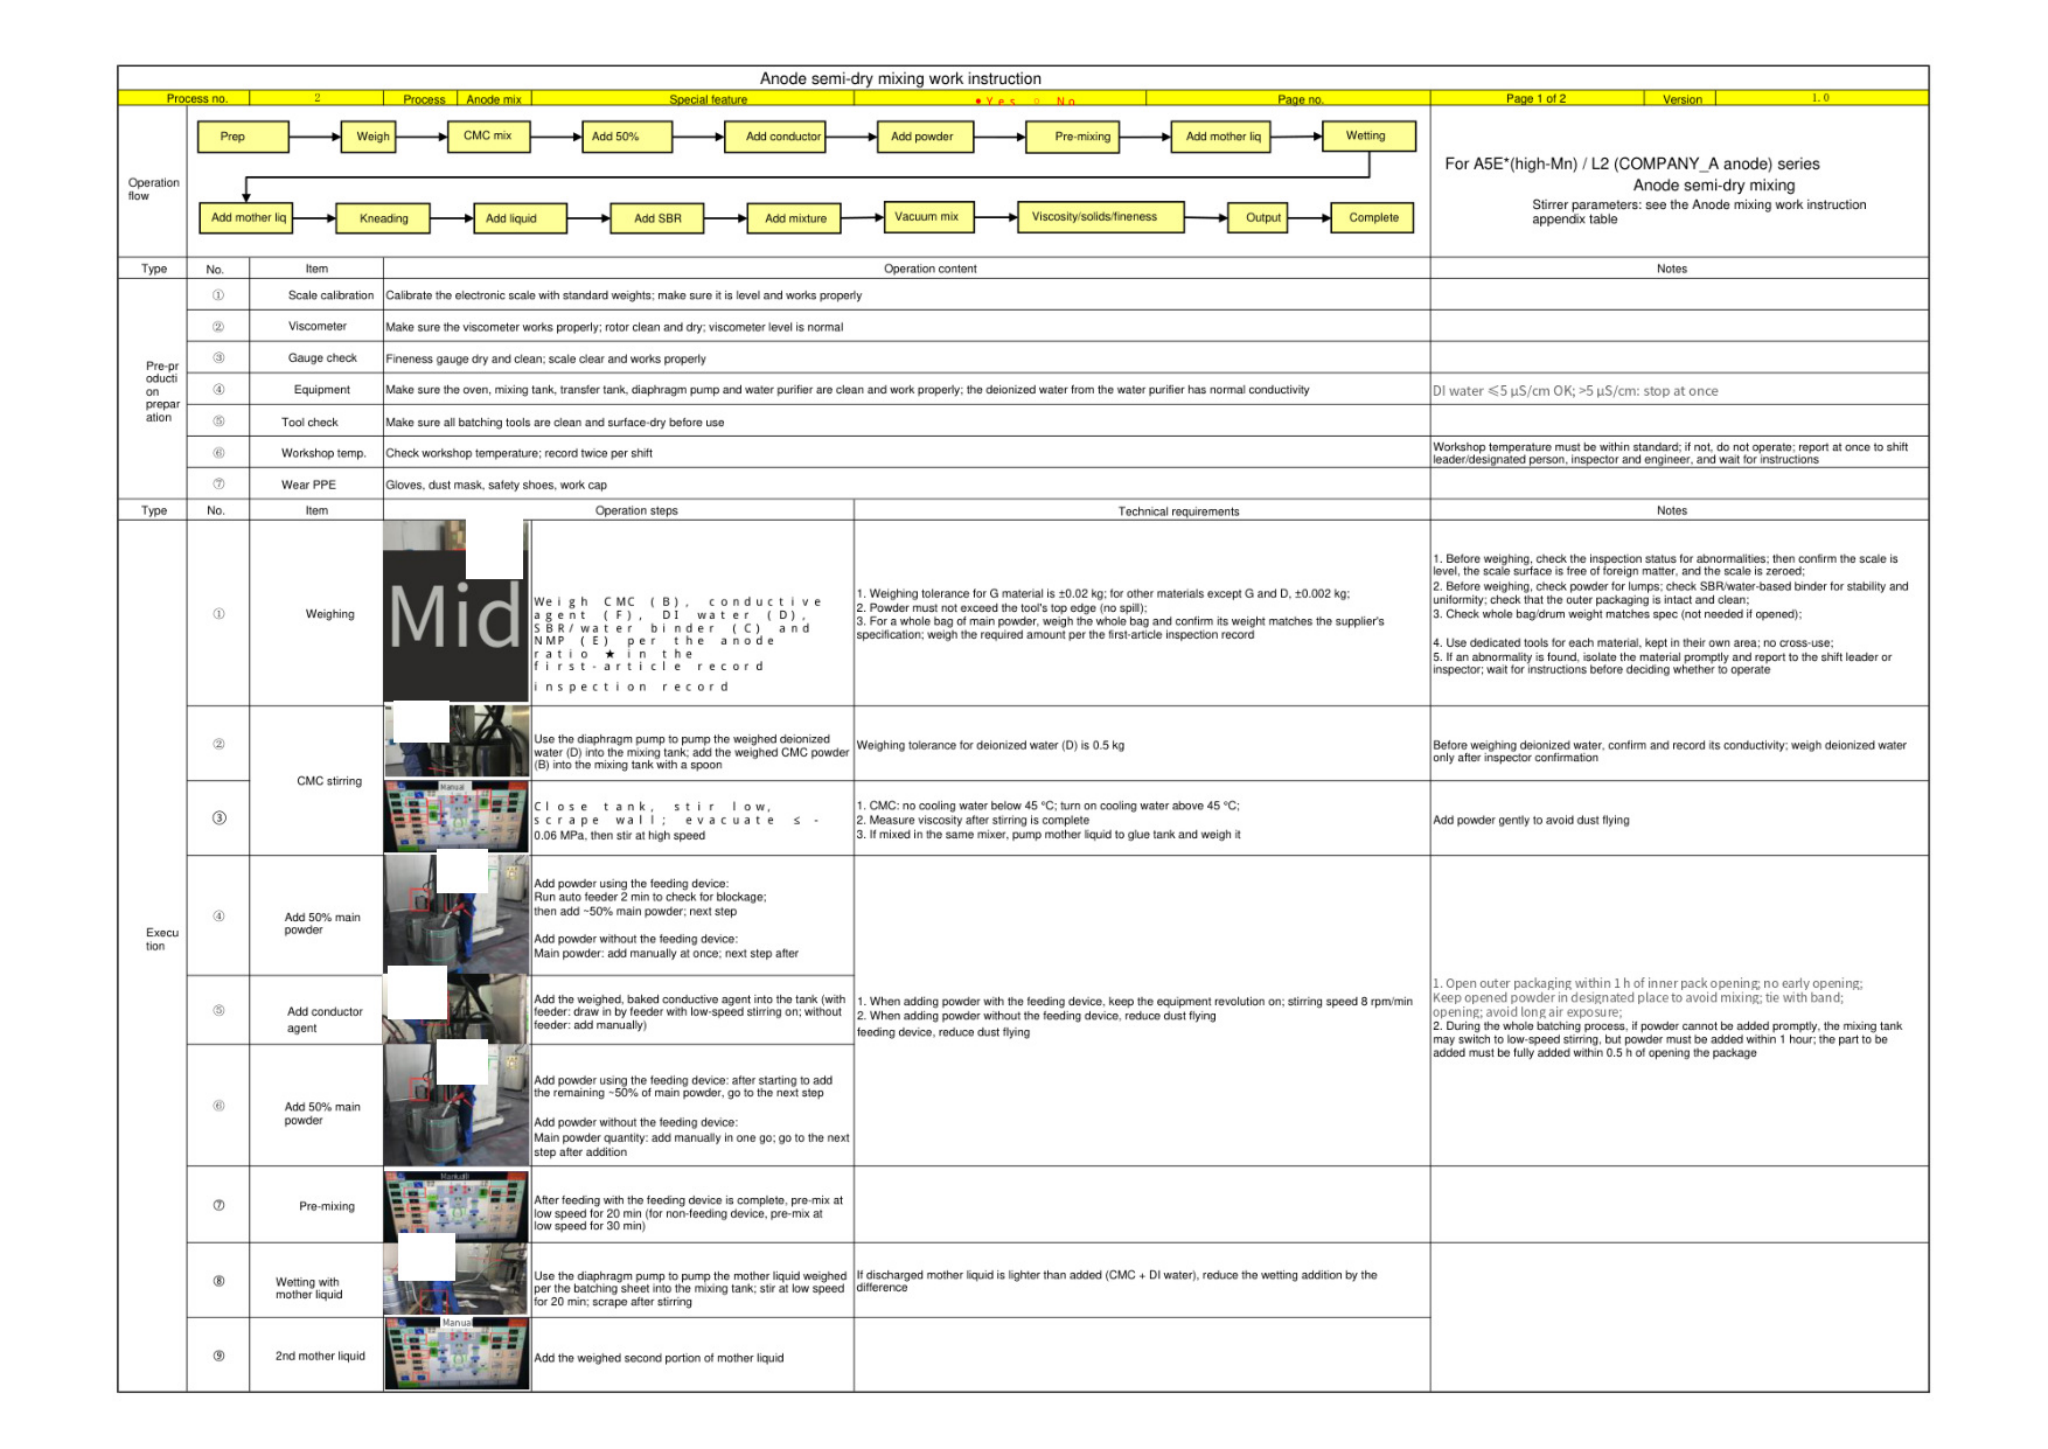# Anode semi-dry mixing work instruction

| Process no. | 2 | Process | Anode mix | Special feature | • Yes ○ No | Page no. | Page 1 of 2 | Version | 1.0 |
|---|---|---|---|---|---|---|---|---|---|

**Operation flow**

Prep → Weigh → CMC mix → Add 50% → Add conductor → Add powder → Pre-mixing → Add mother liq → Wetting → Add mother liq → Kneading → Add liquid → Add SBR → Add mixture → Vacuum mix → Viscosity/solids/fineness → Output → Complete

For A5E*(high-Mn) / L2 (COMPANY_A anode) series
Anode semi-dry mixing
Stirrer parameters: see the Anode mixing work instruction appendix table

| Type | No. | Item | Operation content | Notes |
|---|---|---|---|---|
| Pre-production preparation | ① | Scale calibration | Calibrate the electronic scale with standard weights; make sure it is level and works properly | |
| | ② | Viscometer | Make sure the viscometer works properly; rotor clean and dry; viscometer level is normal | |
| | ③ | Gauge check | Fineness gauge dry and clean; scale clear and works properly | |
| | ④ | Equipment | Make sure the oven, mixing tank, transfer tank, diaphragm pump and water purifier are clean and work properly; the deionized water from the water purifier has normal conductivity | DI water ≤5 µS/cm OK; >5 µS/cm: stop at once |
| | ⑤ | Tool check | Make sure all batching tools are clean and surface-dry before use | |
| | ⑥ | Workshop temp. | Check workshop temperature; record twice per shift | Workshop temperature must be within standard; if not, do not operate; report at once to shift leader/designated person, inspector and engineer, and wait for instructions |
| | ⑦ | Wear PPE | Gloves, dust mask, safety shoes, work cap | |

| Type | No. | Item | Operation steps | Technical requirements | Notes |
|---|---|---|---|---|---|
| Execution | ① | Weighing | Mid<br>Weigh CMC (B), conductive agent (F), DI water (D), SBR/water binder (C) and NMP (E) per the anode ratio ★ in the first-article record<br>inspection record | 1. Weighing tolerance for G material is ±0.02 kg; for other materials except G and D, ±0.002 kg;<br>2. Powder must not exceed the tool's top edge (no spill);<br>3. For a whole bag of main powder, weigh the whole bag and confirm its weight matches the supplier's specification; weigh the required amount per the first-article inspection record | 1. Before weighing, check the inspection status for abnormalities; then confirm the scale is level, the scale surface is free of foreign matter, and the scale is zeroed;<br>2. Before weighing, check powder for lumps; check SBR/water-based binder for stability and uniformity; check that the outer packaging is intact and clean;<br>3. Check whole bag/drum weight matches spec (not needed if opened);<br>4. Use dedicated tools for each material, kept in their own area; no cross-use;<br>5. If an abnormality is found, isolate the material promptly and report to the shift leader or inspector; wait for instructions before deciding whether to operate |
| | ② | CMC stirring | Use the diaphragm pump to pump the weighed deionized water (D) into the mixing tank; add the weighed CMC powder (B) into the mixing tank with a spoon | Weighing tolerance for deionized water (D) is 0.5 kg | Before weighing deionized water, confirm and record its conductivity; weigh deionized water only after inspector confirmation |
| | ③ | | Manual<br>Close tank, stir low, scrape wall; evacuate ≤ -0.06 MPa, then stir at high speed | 1. CMC: no cooling water below 45 °C; turn on cooling water above 45 °C;<br>2. Measure viscosity after stirring is complete<br>3. If mixed in the same mixer, pump mother liquid to glue tank and weigh it | Add powder gently to avoid dust flying |
| | ④ | Add 50% main powder | Add powder using the feeding device:<br>Run auto feeder 2 min to check for blockage;<br>then add ~50% main powder; next step<br><br>Add powder without the feeding device:<br>Main powder: add manually at once; next step after | | |
| | ⑤ | Add conductor agent | Add the weighed, baked conductive agent into the tank (with feeder: draw in by feeder with low-speed stirring on; without feeder: add manually) | 1. When adding powder with the feeding device, keep the equipment revolution on; stirring speed 8 rpm/min<br>2. When adding powder without the feeding device, reduce dust flying<br>feeding device, reduce dust flying | 1. Open outer packaging within 1 h of inner pack opening; no early opening;<br>Keep opened powder in designated place to avoid mixing; tie with band;<br>opening; avoid long air exposure;<br>2. During the whole batching process, if powder cannot be added promptly, the mixing tank may switch to low-speed stirring, but powder must be added within 1 hour; the part to be added must be fully added within 0.5 h of opening the package |
| | ⑥ | Add 50% main powder | Add powder using the feeding device: after starting to add the remaining ~50% of main powder, go to the next step<br><br>Add powder without the feeding device:<br>Main powder quantity: add manually in one go; go to the next step after addition | | |
| | ⑦ | Pre-mixing | Manual<br>After feeding with the feeding device is complete, pre-mix at low speed for 20 min (for non-feeding device, pre-mix at low speed for 30 min) | | |
| | ⑧ | Wetting with mother liquid | Use the diaphragm pump to pump the mother liquid weighed per the batching sheet into the mixing tank; stir at low speed for 20 min; scrape after stirring | If discharged mother liquid is lighter than added (CMC + DI water), reduce the wetting addition by the difference | |
| | ⑨ | 2nd mother liquid | Manual<br>Add the weighed second portion of mother liquid | | |
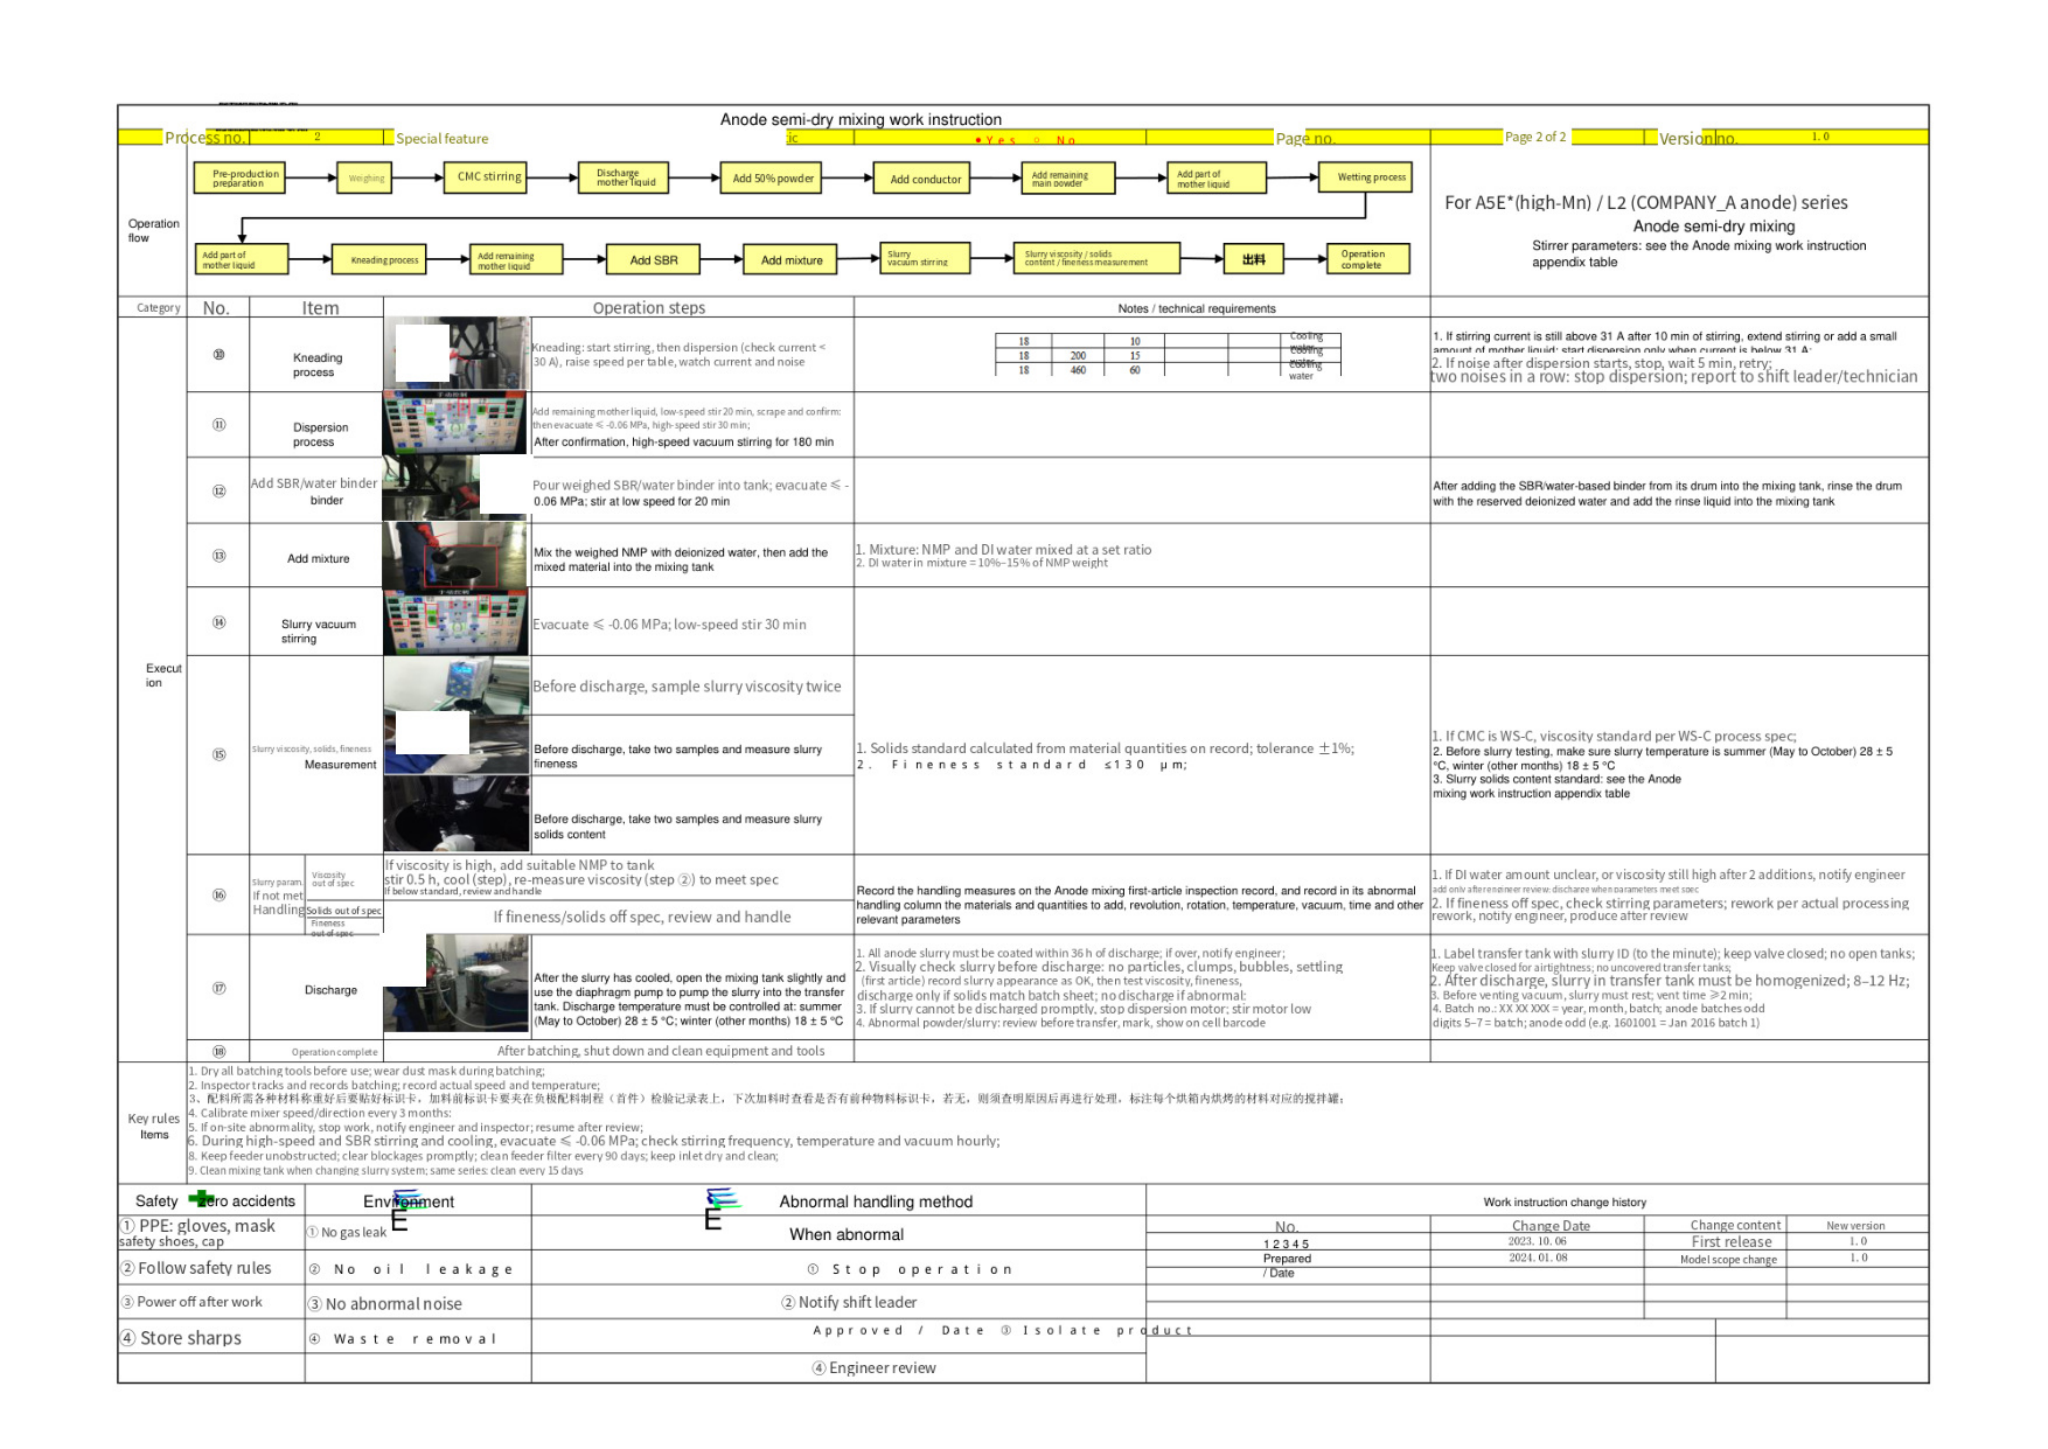# Anode semi-dry mixing work instruction

| Process no. | 2 | Special feature | ic | ● Yes ○ No | Page no. | Page 2 of 2 | Version no. | 1.0 |
|---|---|---|---|---|---|---|---|---|

**Operation flow**

Pre-production preparation → Weighing → CMC stirring → Discharge mother liquid → Add 50% powder → Add conductor → Add remaining main powder → Add part of mother liquid → Wetting process → Add part of mother liquid → Kneading process → Add remaining mother liquid → Add SBR → Add mixture → Slurry vacuum stirring → Slurry viscosity / solids content / fineness measurement → 出料 → Operation complete

For A5E*(high-Mn) / L2 (COMPANY_A anode) series
Anode semi-dry mixing
Stirrer parameters: see the Anode mixing work instruction appendix table

| Category | No. | Item | Operation steps | Notes / technical requirements | |
|---|---|---|---|---|---|
| Execution | ⑩ | Kneading process | Kneading: start stirring, then dispersion (check current < 30 A), raise speed per table, watch current and noise | 18 \| \| 10 \| Cooling water<br>18 \| 200 \| 15 \| Cooling water<br>18 \| 460 \| 60 \| Cooling water | 1. If stirring current is still above 31 A after 10 min of stirring, extend stirring or add a small amount of mother liquid; start dispersion only when current is below 31 A;<br>2. If noise after dispersion starts, stop, wait 5 min, retry; two noises in a row: stop dispersion; report to shift leader/technician |
| | ⑪ | Dispersion process | Add remaining mother liquid, low-speed stir 20 min, scrape and confirm; then evacuate ≤ -0.06 MPa, high-speed stir 30 min;<br>After confirmation, high-speed vacuum stirring for 180 min | | |
| | ⑫ | Add SBR/water binder binder | Pour weighed SBR/water binder into tank; evacuate ≤ -0.06 MPa; stir at low speed for 20 min | | After adding the SBR/water-based binder from its drum into the mixing tank, rinse the drum with the reserved deionized water and add the rinse liquid into the mixing tank |
| | ⑬ | Add mixture | Mix the weighed NMP with deionized water, then add the mixed material into the mixing tank | 1. Mixture: NMP and DI water mixed at a set ratio<br>2. DI water in mixture = 10%–15% of NMP weight | |
| | ⑭ | Slurry vacuum stirring | Evacuate ≤ -0.06 MPa; low-speed stir 30 min | | |
| | ⑮ | Slurry viscosity, solids, fineness Measurement | Before discharge, sample slurry viscosity twice<br>Before discharge, take two samples and measure slurry fineness<br>Before discharge, take two samples and measure slurry solids content | 1. Solids standard calculated from material quantities on record; tolerance ±1%;<br>2. Fineness standard ≤130 μm; | 1. If CMC is WS-C, viscosity standard per WS-C process spec;<br>2. Before slurry testing, make sure slurry temperature is summer (May to October) 28 ± 5 °C, winter (other months) 18 ± 5 °C<br>3. Slurry solids content standard: see the Anode mixing work instruction appendix table |
| | ⑯ | Slurry param. If not met Handling — Viscosity out of spec | If viscosity is high, add suitable NMP to tank stir 0.5 h, cool (step), re-measure viscosity (step ②) to meet spec<br>If below standard, review and handle | Record the handling measures on the Anode mixing first-article inspection record, and record in its abnormal handling column the materials and quantities to add, revolution, rotation, temperature, vacuum, time and other relevant parameters | 1. If DI water amount unclear, or viscosity still high after 2 additions, notify engineer<br>add only after engineer review; discharge when parameters meet spec<br>2. If fineness off spec, check stirring parameters; rework per actual processing<br>rework, notify engineer, produce after review |
| | | Solids out of spec / Fineness out of spec | If fineness/solids off spec, review and handle | | |
| | ⑰ | Discharge | After the slurry has cooled, open the mixing tank slightly and use the diaphragm pump to pump the slurry into the transfer tank. Discharge temperature must be controlled at: summer (May to October) 28 ± 5 °C; winter (other months) 18 ± 5 °C | 1. All anode slurry must be coated within 36 h of discharge; if over, notify engineer;<br>2. Visually check slurry before discharge: no particles, clumps, bubbles, settling (first article) record slurry appearance as OK, then test viscosity, fineness, discharge only if solids match batch sheet; no discharge if abnormal:<br>3. If slurry cannot be discharged promptly, stop dispersion motor; stir motor low<br>4. Abnormal powder/slurry: review before transfer, mark, show on cell barcode | 1. Label transfer tank with slurry ID (to the minute); keep valve closed; no open tanks;<br>Keep valve closed for airtightness; no uncovered transfer tanks;<br>2. After discharge, slurry in transfer tank must be homogenized; 8–12 Hz;<br>3. Before venting vacuum, slurry must rest; vent time ≥2 min;<br>4. Batch no.: XX XX XXX = year, month, batch; anode batches odd digits 5–7 = batch; anode odd (e.g. 1601001 = Jan 2016 batch 1) |
| | ⑱ | Operation complete | After batching, shut down and clean equipment and tools | | |

**Key rules Items**

1. Dry all batching tools before use; wear dust mask during batching;
2. Inspector tracks and records batching; record actual speed and temperature;
3、配料所需各种材料称重好后要贴好标识卡，加料前标识卡要夹在负极配料制程（首件）检验记录表上，下次加料时查看是否有前种物料标识卡，若无，则须查明原因后再进行处理，标注每个烘箱内烘烤的材料对应的搅拌罐；
4. Calibrate mixer speed/direction every 3 months:
5. If on-site abnormality, stop work, notify engineer and inspector; resume after review;
6. During high-speed and SBR stirring and cooling, evacuate ≤ -0.06 MPa; check stirring frequency, temperature and vacuum hourly;
8. Keep feeder unobstructed; clear blockages promptly; clean feeder filter every 90 days; keep inlet dry and clean;
9. Clean mixing tank when changing slurry system; same series: clean every 15 days

| Safety Zero accidents | Environment | Abnormal handling method |
|---|---|---|
| ① PPE: gloves, mask safety shoes, cap | ① No gas leak | When abnormal |
| ② Follow safety rules | ② No oil leakage | ① Stop operation |
| ③ Power off after work | ③ No abnormal noise | ② Notify shift leader |
| ④ Store sharps | ④ Waste removal | ③ Isolate product |
| | | ④ Engineer review |

**Work instruction change history**

| No. | Change Date | Change content | New version |
|---|---|---|---|
| 1 2 3 4 5 | 2023. 10. 06 | First release | 1.0 |
| | 2024. 01. 08 | Model scope change | 1.0 |

Prepared / Date

Approved / Date